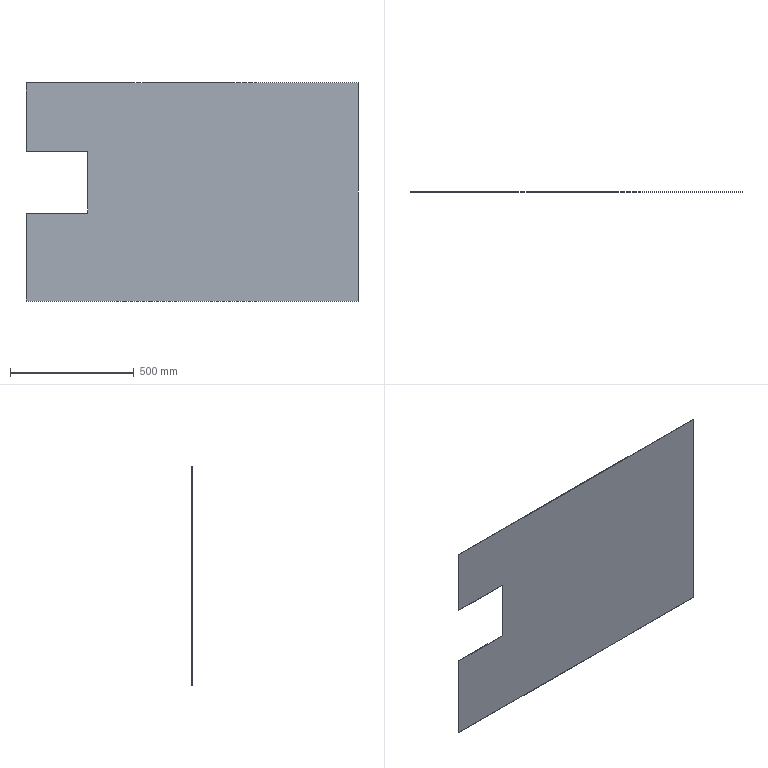Part | STEP file | Sealing plate 1 | 1 solid | 10 faces | box 1340 x 2 x 880 mm | volume 2233400 mm3 | plane 10
STEP:
#1=CARTESIAN_POINT('',(0.,0.,0.));
#2=DIRECTION('',(0.,0.,1.));
#3=DIRECTION('',(1.,0.,0.));
#4=AXIS2_PLACEMENT_3D('',#1,#2,#3);
#5=CARTESIAN_POINT('',(0.,0.,0.));
#6=VERTEX_POINT('',#5);
#7=CARTESIAN_POINT('',(0.,0.,355.));
#8=VERTEX_POINT('',#7);
#9=CARTESIAN_POINT('',(0.,0.,0.));
#10=DIRECTION('',(0.,0.,1.));
#11=VECTOR('',#10,1.);
#12=LINE('',#9,#11);
#13=CARTESIAN_POINT('',(0.,2.,0.));
#14=DIRECTION('',(1.,0.,0.));
#15=DIRECTION('',(0.,0.,-1.));
#16=AXIS2_PLACEMENT_3D('',#13,#14,#15);
#17=PLANE('',#16);
#18=CARTESIAN_POINT('',(0.,-2.));
#19=DIRECTION('',(-1.,0.));
#20=VECTOR('',#19,1.);
#21=LINE('',#18,#20);
#22=(GEOMETRIC_REPRESENTATION_CONTEXT(2)PARAMETRIC_REPRESENTATION_CONTEXT()REPRESENTATION_CONTEXT('',''));
#23=DEFINITIONAL_REPRESENTATION('',(#21),#22);
#24=PCURVE('',#17,#23);
#25=CARTESIAN_POINT('',(0.,0.,0.));
#26=DIRECTION('',(0.,1.,0.));
#27=DIRECTION('',(0.,0.,1.));
#28=AXIS2_PLACEMENT_3D('',#25,#26,#27);
#29=PLANE('',#28);
#30=CARTESIAN_POINT('',(0.,0.));
#31=DIRECTION('',(1.,0.));
#32=VECTOR('',#31,1.);
#33=LINE('',#30,#32);
#34=(GEOMETRIC_REPRESENTATION_CONTEXT(2)PARAMETRIC_REPRESENTATION_CONTEXT()REPRESENTATION_CONTEXT('',''));
#35=DEFINITIONAL_REPRESENTATION('',(#33),#34);
#36=PCURVE('',#29,#35);
#37=SURFACE_CURVE('',#12,(#24,#36),.PCURVE_S1.);
#38=EDGE_CURVE('',#6,#8,#37,.T.);
#39=ORIENTED_EDGE('',*,*,#38,.T.);
#40=CARTESIAN_POINT('',(0.,2.,355.));
#41=VERTEX_POINT('',#40);
#42=CARTESIAN_POINT('',(0.,0.,355.));
#43=DIRECTION('',(0.,1.,0.));
#44=VECTOR('',#43,1.);
#45=LINE('',#42,#44);
#46=CARTESIAN_POINT('',(-355.,-2.));
#47=DIRECTION('',(0.,1.));
#48=VECTOR('',#47,1.);
#49=LINE('',#46,#48);
#50=(GEOMETRIC_REPRESENTATION_CONTEXT(2)PARAMETRIC_REPRESENTATION_CONTEXT()REPRESENTATION_CONTEXT('',''));
#51=DEFINITIONAL_REPRESENTATION('',(#49),#50);
#52=PCURVE('',#17,#51);
#53=CARTESIAN_POINT('',(0.,0.,355.));
#54=DIRECTION('',(0.,0.,-1.));
#55=DIRECTION('',(-1.,0.,0.));
#56=AXIS2_PLACEMENT_3D('',#53,#54,#55);
#57=PLANE('',#56);
#58=CARTESIAN_POINT('',(0.,0.));
#59=DIRECTION('',(0.,1.));
#60=VECTOR('',#59,1.);
#61=LINE('',#58,#60);
#62=(GEOMETRIC_REPRESENTATION_CONTEXT(2)PARAMETRIC_REPRESENTATION_CONTEXT()REPRESENTATION_CONTEXT('',''));
#63=DEFINITIONAL_REPRESENTATION('',(#61),#62);
#64=PCURVE('',#57,#63);
#65=SURFACE_CURVE('',#45,(#52,#64),.PCURVE_S1.);
#66=EDGE_CURVE('',#8,#41,#65,.T.);
#67=ORIENTED_EDGE('',*,*,#66,.T.);
#68=CARTESIAN_POINT('',(0.,2.,0.));
#69=VERTEX_POINT('',#68);
#70=CARTESIAN_POINT('',(0.,2.,0.));
#71=DIRECTION('',(0.,0.,1.));
#72=VECTOR('',#71,1.);
#73=LINE('',#70,#72);
#74=CARTESIAN_POINT('',(0.,0.));
#75=DIRECTION('',(-1.,0.));
#76=VECTOR('',#75,1.);
#77=LINE('',#74,#76);
#78=(GEOMETRIC_REPRESENTATION_CONTEXT(2)PARAMETRIC_REPRESENTATION_CONTEXT()REPRESENTATION_CONTEXT('',''));
#79=DEFINITIONAL_REPRESENTATION('',(#77),#78);
#80=PCURVE('',#17,#79);
#81=CARTESIAN_POINT('',(0.,2.,0.));
#82=DIRECTION('',(0.,1.,0.));
#83=DIRECTION('',(0.,0.,1.));
#84=AXIS2_PLACEMENT_3D('',#81,#82,#83);
#85=PLANE('',#84);
#86=CARTESIAN_POINT('',(0.,0.));
#87=DIRECTION('',(1.,0.));
#88=VECTOR('',#87,1.);
#89=LINE('',#86,#88);
#90=(GEOMETRIC_REPRESENTATION_CONTEXT(2)PARAMETRIC_REPRESENTATION_CONTEXT()REPRESENTATION_CONTEXT('',''));
#91=DEFINITIONAL_REPRESENTATION('',(#89),#90);
#92=PCURVE('',#85,#91);
#93=SURFACE_CURVE('',#73,(#80,#92),.PCURVE_S1.);
#94=EDGE_CURVE('',#69,#41,#93,.T.);
#95=ORIENTED_EDGE('',*,*,#94,.F.);
#96=CARTESIAN_POINT('',(0.,2.,0.));
#97=DIRECTION('',(0.,-1.,0.));
#98=VECTOR('',#97,1.);
#99=LINE('',#96,#98);
#100=CARTESIAN_POINT('',(0.,0.));
#101=DIRECTION('',(0.,-1.));
#102=VECTOR('',#101,1.);
#103=LINE('',#100,#102);
#104=(GEOMETRIC_REPRESENTATION_CONTEXT(2)PARAMETRIC_REPRESENTATION_CONTEXT()REPRESENTATION_CONTEXT('',''));
#105=DEFINITIONAL_REPRESENTATION('',(#103),#104);
#106=PCURVE('',#17,#105);
#107=CARTESIAN_POINT('',(0.,2.,0.));
#108=DIRECTION('',(0.,0.,1.));
#109=DIRECTION('',(1.,0.,0.));
#110=AXIS2_PLACEMENT_3D('',#107,#108,#109);
#111=PLANE('',#110);
#112=CARTESIAN_POINT('',(0.,0.));
#113=DIRECTION('',(0.,-1.));
#114=VECTOR('',#113,1.);
#115=LINE('',#112,#114);
#116=(GEOMETRIC_REPRESENTATION_CONTEXT(2)PARAMETRIC_REPRESENTATION_CONTEXT()REPRESENTATION_CONTEXT('',''));
#117=DEFINITIONAL_REPRESENTATION('',(#115),#116);
#118=PCURVE('',#111,#117);
#119=SURFACE_CURVE('',#99,(#106,#118),.PCURVE_S1.);
#120=EDGE_CURVE('',#69,#6,#119,.T.);
#121=ORIENTED_EDGE('',*,*,#120,.T.);
#122=EDGE_LOOP('',(#39,#67,#95,#121));
#123=FACE_BOUND('',#122,.T.);
#124=ADVANCED_FACE('',(#123),#17,.F.);
#125=CARTESIAN_POINT('',(0.,2.,605.));
#126=VERTEX_POINT('',#125);
#127=CARTESIAN_POINT('',(0.,2.,880.));
#128=VERTEX_POINT('',#127);
#129=CARTESIAN_POINT('',(0.,2.,0.));
#130=DIRECTION('',(0.,0.,1.));
#131=VECTOR('',#130,1.);
#132=LINE('',#129,#131);
#133=CARTESIAN_POINT('',(0.,2.,0.));
#134=DIRECTION('',(1.,0.,0.));
#135=DIRECTION('',(0.,0.,-1.));
#136=AXIS2_PLACEMENT_3D('',#133,#134,#135);
#137=PLANE('',#136);
#138=CARTESIAN_POINT('',(0.,0.));
#139=DIRECTION('',(-1.,0.));
#140=VECTOR('',#139,1.);
#141=LINE('',#138,#140);
#142=(GEOMETRIC_REPRESENTATION_CONTEXT(2)PARAMETRIC_REPRESENTATION_CONTEXT()REPRESENTATION_CONTEXT('',''));
#143=DEFINITIONAL_REPRESENTATION('',(#141),#142);
#144=PCURVE('',#137,#143);
#145=CARTESIAN_POINT('',(0.,0.));
#146=DIRECTION('',(1.,0.));
#147=VECTOR('',#146,1.);
#148=LINE('',#145,#147);
#149=(GEOMETRIC_REPRESENTATION_CONTEXT(2)PARAMETRIC_REPRESENTATION_CONTEXT()REPRESENTATION_CONTEXT('',''));
#150=DEFINITIONAL_REPRESENTATION('',(#148),#149);
#151=PCURVE('',#85,#150);
#152=SURFACE_CURVE('',#132,(#144,#151),.PCURVE_S1.);
#153=EDGE_CURVE('',#126,#128,#152,.T.);
#154=ORIENTED_EDGE('',*,*,#153,.F.);
#155=CARTESIAN_POINT('',(0.,0.,605.));
#156=VERTEX_POINT('',#155);
#157=CARTESIAN_POINT('',(0.,0.,605.));
#158=DIRECTION('',(0.,1.,0.));
#159=VECTOR('',#158,1.);
#160=LINE('',#157,#159);
#161=CARTESIAN_POINT('',(-605.,-2.));
#162=DIRECTION('',(0.,1.));
#163=VECTOR('',#162,1.);
#164=LINE('',#161,#163);
#165=(GEOMETRIC_REPRESENTATION_CONTEXT(2)PARAMETRIC_REPRESENTATION_CONTEXT()REPRESENTATION_CONTEXT('',''));
#166=DEFINITIONAL_REPRESENTATION('',(#164),#165);
#167=PCURVE('',#137,#166);
#168=CARTESIAN_POINT('',(0.,0.,605.));
#169=DIRECTION('',(0.,0.,1.));
#170=DIRECTION('',(1.,0.,0.));
#171=AXIS2_PLACEMENT_3D('',#168,#169,#170);
#172=PLANE('',#171);
#173=CARTESIAN_POINT('',(0.,0.));
#174=DIRECTION('',(0.,1.));
#175=VECTOR('',#174,1.);
#176=LINE('',#173,#175);
#177=(GEOMETRIC_REPRESENTATION_CONTEXT(2)PARAMETRIC_REPRESENTATION_CONTEXT()REPRESENTATION_CONTEXT('',''));
#178=DEFINITIONAL_REPRESENTATION('',(#176),#177);
#179=PCURVE('',#172,#178);
#180=SURFACE_CURVE('',#160,(#167,#179),.PCURVE_S1.);
#181=EDGE_CURVE('',#156,#126,#180,.T.);
#182=ORIENTED_EDGE('',*,*,#181,.F.);
#183=CARTESIAN_POINT('',(0.,0.,880.));
#184=VERTEX_POINT('',#183);
#185=CARTESIAN_POINT('',(0.,0.,0.));
#186=DIRECTION('',(0.,0.,1.));
#187=VECTOR('',#186,1.);
#188=LINE('',#185,#187);
#189=CARTESIAN_POINT('',(0.,-2.));
#190=DIRECTION('',(-1.,0.));
#191=VECTOR('',#190,1.);
#192=LINE('',#189,#191);
#193=(GEOMETRIC_REPRESENTATION_CONTEXT(2)PARAMETRIC_REPRESENTATION_CONTEXT()REPRESENTATION_CONTEXT('',''));
#194=DEFINITIONAL_REPRESENTATION('',(#192),#193);
#195=PCURVE('',#137,#194);
#196=CARTESIAN_POINT('',(0.,0.));
#197=DIRECTION('',(1.,0.));
#198=VECTOR('',#197,1.);
#199=LINE('',#196,#198);
#200=(GEOMETRIC_REPRESENTATION_CONTEXT(2)PARAMETRIC_REPRESENTATION_CONTEXT()REPRESENTATION_CONTEXT('',''));
#201=DEFINITIONAL_REPRESENTATION('',(#199),#200);
#202=PCURVE('',#29,#201);
#203=SURFACE_CURVE('',#188,(#195,#202),.PCURVE_S1.);
#204=EDGE_CURVE('',#156,#184,#203,.T.);
#205=ORIENTED_EDGE('',*,*,#204,.T.);
#206=CARTESIAN_POINT('',(0.,2.,880.));
#207=DIRECTION('',(0.,-1.,0.));
#208=VECTOR('',#207,1.);
#209=LINE('',#206,#208);
#210=CARTESIAN_POINT('',(-880.,0.));
#211=DIRECTION('',(0.,-1.));
#212=VECTOR('',#211,1.);
#213=LINE('',#210,#212);
#214=(GEOMETRIC_REPRESENTATION_CONTEXT(2)PARAMETRIC_REPRESENTATION_CONTEXT()REPRESENTATION_CONTEXT('',''));
#215=DEFINITIONAL_REPRESENTATION('',(#213),#214);
#216=PCURVE('',#137,#215);
#217=CARTESIAN_POINT('',(0.,2.,880.));
#218=DIRECTION('',(0.,0.,-1.));
#219=DIRECTION('',(-1.,0.,0.));
#220=AXIS2_PLACEMENT_3D('',#217,#218,#219);
#221=PLANE('',#220);
#222=CARTESIAN_POINT('',(0.,0.));
#223=DIRECTION('',(0.,-1.));
#224=VECTOR('',#223,1.);
#225=LINE('',#222,#224);
#226=(GEOMETRIC_REPRESENTATION_CONTEXT(2)PARAMETRIC_REPRESENTATION_CONTEXT()REPRESENTATION_CONTEXT('',''));
#227=DEFINITIONAL_REPRESENTATION('',(#225),#226);
#228=PCURVE('',#221,#227);
#229=SURFACE_CURVE('',#209,(#216,#228),.PCURVE_S1.);
#230=EDGE_CURVE('',#128,#184,#229,.T.);
#231=ORIENTED_EDGE('',*,*,#230,.F.);
#232=EDGE_LOOP('',(#154,#182,#205,#231));
#233=FACE_BOUND('',#232,.T.);
#234=ADVANCED_FACE('',(#233),#137,.F.);
#235=CARTESIAN_POINT('',(1340.,0.,880.));
#236=VERTEX_POINT('',#235);
#237=CARTESIAN_POINT('',(0.,0.,880.));
#238=DIRECTION('',(1.,0.,0.));
#239=VECTOR('',#238,1.);
#240=LINE('',#237,#239);
#241=CARTESIAN_POINT('',(0.,-2.));
#242=DIRECTION('',(-1.,0.));
#243=VECTOR('',#242,1.);
#244=LINE('',#241,#243);
#245=(GEOMETRIC_REPRESENTATION_CONTEXT(2)PARAMETRIC_REPRESENTATION_CONTEXT()REPRESENTATION_CONTEXT('',''));
#246=DEFINITIONAL_REPRESENTATION('',(#244),#245);
#247=PCURVE('',#221,#246);
#248=CARTESIAN_POINT('',(880.,0.));
#249=DIRECTION('',(0.,1.));
#250=VECTOR('',#249,1.);
#251=LINE('',#248,#250);
#252=(GEOMETRIC_REPRESENTATION_CONTEXT(2)PARAMETRIC_REPRESENTATION_CONTEXT()REPRESENTATION_CONTEXT('',''));
#253=DEFINITIONAL_REPRESENTATION('',(#251),#252);
#254=PCURVE('',#29,#253);
#255=SURFACE_CURVE('',#240,(#247,#254),.PCURVE_S1.);
#256=EDGE_CURVE('',#184,#236,#255,.T.);
#257=ORIENTED_EDGE('',*,*,#256,.T.);
#258=CARTESIAN_POINT('',(1340.,2.,880.));
#259=VERTEX_POINT('',#258);
#260=CARTESIAN_POINT('',(1340.,2.,880.));
#261=DIRECTION('',(0.,-1.,0.));
#262=VECTOR('',#261,1.);
#263=LINE('',#260,#262);
#264=CARTESIAN_POINT('',(-1340.,0.));
#265=DIRECTION('',(0.,-1.));
#266=VECTOR('',#265,1.);
#267=LINE('',#264,#266);
#268=(GEOMETRIC_REPRESENTATION_CONTEXT(2)PARAMETRIC_REPRESENTATION_CONTEXT()REPRESENTATION_CONTEXT('',''));
#269=DEFINITIONAL_REPRESENTATION('',(#267),#268);
#270=PCURVE('',#221,#269);
#271=CARTESIAN_POINT('',(1340.,2.,0.));
#272=DIRECTION('',(-1.,0.,0.));
#273=DIRECTION('',(0.,0.,1.));
#274=AXIS2_PLACEMENT_3D('',#271,#272,#273);
#275=PLANE('',#274);
#276=CARTESIAN_POINT('',(880.,0.));
#277=DIRECTION('',(0.,-1.));
#278=VECTOR('',#277,1.);
#279=LINE('',#276,#278);
#280=(GEOMETRIC_REPRESENTATION_CONTEXT(2)PARAMETRIC_REPRESENTATION_CONTEXT()REPRESENTATION_CONTEXT('',''));
#281=DEFINITIONAL_REPRESENTATION('',(#279),#280);
#282=PCURVE('',#275,#281);
#283=SURFACE_CURVE('',#263,(#270,#282),.PCURVE_S1.);
#284=EDGE_CURVE('',#259,#236,#283,.T.);
#285=ORIENTED_EDGE('',*,*,#284,.F.);
#286=CARTESIAN_POINT('',(0.,2.,880.));
#287=DIRECTION('',(1.,0.,0.));
#288=VECTOR('',#287,1.);
#289=LINE('',#286,#288);
#290=CARTESIAN_POINT('',(0.,0.));
#291=DIRECTION('',(-1.,0.));
#292=VECTOR('',#291,1.);
#293=LINE('',#290,#292);
#294=(GEOMETRIC_REPRESENTATION_CONTEXT(2)PARAMETRIC_REPRESENTATION_CONTEXT()REPRESENTATION_CONTEXT('',''));
#295=DEFINITIONAL_REPRESENTATION('',(#293),#294);
#296=PCURVE('',#221,#295);
#297=CARTESIAN_POINT('',(880.,0.));
#298=DIRECTION('',(0.,1.));
#299=VECTOR('',#298,1.);
#300=LINE('',#297,#299);
#301=(GEOMETRIC_REPRESENTATION_CONTEXT(2)PARAMETRIC_REPRESENTATION_CONTEXT()REPRESENTATION_CONTEXT('',''));
#302=DEFINITIONAL_REPRESENTATION('',(#300),#301);
#303=PCURVE('',#85,#302);
#304=SURFACE_CURVE('',#289,(#296,#303),.PCURVE_S1.);
#305=EDGE_CURVE('',#128,#259,#304,.T.);
#306=ORIENTED_EDGE('',*,*,#305,.F.);
#307=ORIENTED_EDGE('',*,*,#230,.T.);
#308=EDGE_LOOP('',(#257,#285,#306,#307));
#309=FACE_BOUND('',#308,.T.);
#310=ADVANCED_FACE('',(#309),#221,.F.);
#311=CARTESIAN_POINT('',(1340.,0.,0.));
#312=VERTEX_POINT('',#311);
#313=CARTESIAN_POINT('',(1340.,0.,0.));
#314=DIRECTION('',(0.,0.,-1.));
#315=VECTOR('',#314,1.);
#316=LINE('',#313,#315);
#317=CARTESIAN_POINT('',(0.,-2.));
#318=DIRECTION('',(-1.,0.));
#319=VECTOR('',#318,1.);
#320=LINE('',#317,#319);
#321=(GEOMETRIC_REPRESENTATION_CONTEXT(2)PARAMETRIC_REPRESENTATION_CONTEXT()REPRESENTATION_CONTEXT('',''));
#322=DEFINITIONAL_REPRESENTATION('',(#320),#321);
#323=PCURVE('',#275,#322);
#324=CARTESIAN_POINT('',(0.,1340.));
#325=DIRECTION('',(-1.,0.));
#326=VECTOR('',#325,1.);
#327=LINE('',#324,#326);
#328=(GEOMETRIC_REPRESENTATION_CONTEXT(2)PARAMETRIC_REPRESENTATION_CONTEXT()REPRESENTATION_CONTEXT('',''));
#329=DEFINITIONAL_REPRESENTATION('',(#327),#328);
#330=PCURVE('',#29,#329);
#331=SURFACE_CURVE('',#316,(#323,#330),.PCURVE_S1.);
#332=EDGE_CURVE('',#236,#312,#331,.T.);
#333=ORIENTED_EDGE('',*,*,#332,.T.);
#334=CARTESIAN_POINT('',(1340.,2.,0.));
#335=VERTEX_POINT('',#334);
#336=CARTESIAN_POINT('',(1340.,2.,0.));
#337=DIRECTION('',(0.,-1.,0.));
#338=VECTOR('',#337,1.);
#339=LINE('',#336,#338);
#340=CARTESIAN_POINT('',(0.,0.));
#341=DIRECTION('',(0.,-1.));
#342=VECTOR('',#341,1.);
#343=LINE('',#340,#342);
#344=(GEOMETRIC_REPRESENTATION_CONTEXT(2)PARAMETRIC_REPRESENTATION_CONTEXT()REPRESENTATION_CONTEXT('',''));
#345=DEFINITIONAL_REPRESENTATION('',(#343),#344);
#346=PCURVE('',#275,#345);
#347=CARTESIAN_POINT('',(1340.,0.));
#348=DIRECTION('',(0.,-1.));
#349=VECTOR('',#348,1.);
#350=LINE('',#347,#349);
#351=(GEOMETRIC_REPRESENTATION_CONTEXT(2)PARAMETRIC_REPRESENTATION_CONTEXT()REPRESENTATION_CONTEXT('',''));
#352=DEFINITIONAL_REPRESENTATION('',(#350),#351);
#353=PCURVE('',#111,#352);
#354=SURFACE_CURVE('',#339,(#346,#353),.PCURVE_S1.);
#355=EDGE_CURVE('',#335,#312,#354,.T.);
#356=ORIENTED_EDGE('',*,*,#355,.F.);
#357=CARTESIAN_POINT('',(1340.,2.,0.));
#358=DIRECTION('',(0.,0.,-1.));
#359=VECTOR('',#358,1.);
#360=LINE('',#357,#359);
#361=CARTESIAN_POINT('',(0.,0.));
#362=DIRECTION('',(-1.,0.));
#363=VECTOR('',#362,1.);
#364=LINE('',#361,#363);
#365=(GEOMETRIC_REPRESENTATION_CONTEXT(2)PARAMETRIC_REPRESENTATION_CONTEXT()REPRESENTATION_CONTEXT('',''));
#366=DEFINITIONAL_REPRESENTATION('',(#364),#365);
#367=PCURVE('',#275,#366);
#368=CARTESIAN_POINT('',(0.,1340.));
#369=DIRECTION('',(-1.,0.));
#370=VECTOR('',#369,1.);
#371=LINE('',#368,#370);
#372=(GEOMETRIC_REPRESENTATION_CONTEXT(2)PARAMETRIC_REPRESENTATION_CONTEXT()REPRESENTATION_CONTEXT('',''));
#373=DEFINITIONAL_REPRESENTATION('',(#371),#372);
#374=PCURVE('',#85,#373);
#375=SURFACE_CURVE('',#360,(#367,#374),.PCURVE_S1.);
#376=EDGE_CURVE('',#259,#335,#375,.T.);
#377=ORIENTED_EDGE('',*,*,#376,.F.);
#378=ORIENTED_EDGE('',*,*,#284,.T.);
#379=EDGE_LOOP('',(#333,#356,#377,#378));
#380=FACE_BOUND('',#379,.T.);
#381=ADVANCED_FACE('',(#380),#275,.F.);
#382=CARTESIAN_POINT('',(0.,0.,0.));
#383=DIRECTION('',(-1.,0.,0.));
#384=VECTOR('',#383,1.);
#385=LINE('',#382,#384);
#386=CARTESIAN_POINT('',(0.,-2.));
#387=DIRECTION('',(-1.,0.));
#388=VECTOR('',#387,1.);
#389=LINE('',#386,#388);
#390=(GEOMETRIC_REPRESENTATION_CONTEXT(2)PARAMETRIC_REPRESENTATION_CONTEXT()REPRESENTATION_CONTEXT('',''));
#391=DEFINITIONAL_REPRESENTATION('',(#389),#390);
#392=PCURVE('',#111,#391);
#393=CARTESIAN_POINT('',(0.,0.));
#394=DIRECTION('',(0.,-1.));
#395=VECTOR('',#394,1.);
#396=LINE('',#393,#395);
#397=(GEOMETRIC_REPRESENTATION_CONTEXT(2)PARAMETRIC_REPRESENTATION_CONTEXT()REPRESENTATION_CONTEXT('',''));
#398=DEFINITIONAL_REPRESENTATION('',(#396),#397);
#399=PCURVE('',#29,#398);
#400=SURFACE_CURVE('',#385,(#392,#399),.PCURVE_S1.);
#401=EDGE_CURVE('',#312,#6,#400,.T.);
#402=ORIENTED_EDGE('',*,*,#401,.T.);
#403=ORIENTED_EDGE('',*,*,#120,.F.);
#404=CARTESIAN_POINT('',(0.,2.,0.));
#405=DIRECTION('',(-1.,0.,0.));
#406=VECTOR('',#405,1.);
#407=LINE('',#404,#406);
#408=CARTESIAN_POINT('',(0.,0.));
#409=DIRECTION('',(-1.,0.));
#410=VECTOR('',#409,1.);
#411=LINE('',#408,#410);
#412=(GEOMETRIC_REPRESENTATION_CONTEXT(2)PARAMETRIC_REPRESENTATION_CONTEXT()REPRESENTATION_CONTEXT('',''));
#413=DEFINITIONAL_REPRESENTATION('',(#411),#412);
#414=PCURVE('',#111,#413);
#415=CARTESIAN_POINT('',(0.,0.));
#416=DIRECTION('',(0.,-1.));
#417=VECTOR('',#416,1.);
#418=LINE('',#415,#417);
#419=(GEOMETRIC_REPRESENTATION_CONTEXT(2)PARAMETRIC_REPRESENTATION_CONTEXT()REPRESENTATION_CONTEXT('',''));
#420=DEFINITIONAL_REPRESENTATION('',(#418),#419);
#421=PCURVE('',#85,#420);
#422=SURFACE_CURVE('',#407,(#414,#421),.PCURVE_S1.);
#423=EDGE_CURVE('',#335,#69,#422,.T.);
#424=ORIENTED_EDGE('',*,*,#423,.F.);
#425=ORIENTED_EDGE('',*,*,#355,.T.);
#426=EDGE_LOOP('',(#402,#403,#424,#425));
#427=FACE_BOUND('',#426,.T.);
#428=ADVANCED_FACE('',(#427),#111,.F.);
#429=CARTESIAN_POINT('',(250.,2.,355.));
#430=VERTEX_POINT('',#429);
#431=CARTESIAN_POINT('',(0.,2.,355.));
#432=DIRECTION('',(-1.,0.,0.));
#433=VECTOR('',#432,1.);
#434=LINE('',#431,#433);
#435=CARTESIAN_POINT('',(355.,0.));
#436=DIRECTION('',(0.,-1.));
#437=VECTOR('',#436,1.);
#438=LINE('',#435,#437);
#439=(GEOMETRIC_REPRESENTATION_CONTEXT(2)PARAMETRIC_REPRESENTATION_CONTEXT()REPRESENTATION_CONTEXT('',''));
#440=DEFINITIONAL_REPRESENTATION('',(#438),#439);
#441=PCURVE('',#85,#440);
#442=CARTESIAN_POINT('',(0.,2.));
#443=DIRECTION('',(1.,0.));
#444=VECTOR('',#443,1.);
#445=LINE('',#442,#444);
#446=(GEOMETRIC_REPRESENTATION_CONTEXT(2)PARAMETRIC_REPRESENTATION_CONTEXT()REPRESENTATION_CONTEXT('',''));
#447=DEFINITIONAL_REPRESENTATION('',(#445),#446);
#448=PCURVE('',#57,#447);
#449=SURFACE_CURVE('',#434,(#441,#448),.PCURVE_S1.);
#450=EDGE_CURVE('',#430,#41,#449,.T.);
#451=ORIENTED_EDGE('',*,*,#450,.F.);
#452=CARTESIAN_POINT('',(250.,2.,605.));
#453=VERTEX_POINT('',#452);
#454=CARTESIAN_POINT('',(250.,2.,605.));
#455=DIRECTION('',(0.,0.,-1.));
#456=VECTOR('',#455,1.);
#457=LINE('',#454,#456);
#458=CARTESIAN_POINT('',(605.,250.));
#459=DIRECTION('',(-1.,0.));
#460=VECTOR('',#459,1.);
#461=LINE('',#458,#460);
#462=(GEOMETRIC_REPRESENTATION_CONTEXT(2)PARAMETRIC_REPRESENTATION_CONTEXT()REPRESENTATION_CONTEXT('',''));
#463=DEFINITIONAL_REPRESENTATION('',(#461),#462);
#464=PCURVE('',#85,#463);
#465=CARTESIAN_POINT('',(250.,0.,605.));
#466=DIRECTION('',(1.,0.,0.));
#467=DIRECTION('',(0.,0.,-1.));
#468=AXIS2_PLACEMENT_3D('',#465,#466,#467);
#469=PLANE('',#468);
#470=CARTESIAN_POINT('',(0.,2.));
#471=DIRECTION('',(1.,0.));
#472=VECTOR('',#471,1.);
#473=LINE('',#470,#472);
#474=(GEOMETRIC_REPRESENTATION_CONTEXT(2)PARAMETRIC_REPRESENTATION_CONTEXT()REPRESENTATION_CONTEXT('',''));
#475=DEFINITIONAL_REPRESENTATION('',(#473),#474);
#476=PCURVE('',#469,#475);
#477=SURFACE_CURVE('',#457,(#464,#476),.PCURVE_S1.);
#478=EDGE_CURVE('',#453,#430,#477,.T.);
#479=ORIENTED_EDGE('',*,*,#478,.F.);
#480=CARTESIAN_POINT('',(0.,2.,605.));
#481=DIRECTION('',(1.,0.,0.));
#482=VECTOR('',#481,1.);
#483=LINE('',#480,#482);
#484=CARTESIAN_POINT('',(605.,0.));
#485=DIRECTION('',(0.,1.));
#486=VECTOR('',#485,1.);
#487=LINE('',#484,#486);
#488=(GEOMETRIC_REPRESENTATION_CONTEXT(2)PARAMETRIC_REPRESENTATION_CONTEXT()REPRESENTATION_CONTEXT('',''));
#489=DEFINITIONAL_REPRESENTATION('',(#487),#488);
#490=PCURVE('',#85,#489);
#491=CARTESIAN_POINT('',(0.,2.));
#492=DIRECTION('',(1.,0.));
#493=VECTOR('',#492,1.);
#494=LINE('',#491,#493);
#495=(GEOMETRIC_REPRESENTATION_CONTEXT(2)PARAMETRIC_REPRESENTATION_CONTEXT()REPRESENTATION_CONTEXT('',''));
#496=DEFINITIONAL_REPRESENTATION('',(#494),#495);
#497=PCURVE('',#172,#496);
#498=SURFACE_CURVE('',#483,(#490,#497),.PCURVE_S1.);
#499=EDGE_CURVE('',#126,#453,#498,.T.);
#500=ORIENTED_EDGE('',*,*,#499,.F.);
#501=ORIENTED_EDGE('',*,*,#153,.T.);
#502=ORIENTED_EDGE('',*,*,#305,.T.);
#503=ORIENTED_EDGE('',*,*,#376,.T.);
#504=ORIENTED_EDGE('',*,*,#423,.T.);
#505=ORIENTED_EDGE('',*,*,#94,.T.);
#506=EDGE_LOOP('',(#451,#479,#500,#501,#502,#503,#504,#505));
#507=FACE_BOUND('',#506,.T.);
#508=ADVANCED_FACE('',(#507),#85,.T.);
#509=CARTESIAN_POINT('',(250.,0.,605.));
#510=VERTEX_POINT('',#509);
#511=CARTESIAN_POINT('',(250.,0.,355.));
#512=VERTEX_POINT('',#511);
#513=CARTESIAN_POINT('',(250.,0.,605.));
#514=DIRECTION('',(0.,0.,-1.));
#515=VECTOR('',#514,1.);
#516=LINE('',#513,#515);
#517=CARTESIAN_POINT('',(605.,250.));
#518=DIRECTION('',(-1.,0.));
#519=VECTOR('',#518,1.);
#520=LINE('',#517,#519);
#521=(GEOMETRIC_REPRESENTATION_CONTEXT(2)PARAMETRIC_REPRESENTATION_CONTEXT()REPRESENTATION_CONTEXT('',''));
#522=DEFINITIONAL_REPRESENTATION('',(#520),#521);
#523=PCURVE('',#29,#522);
#524=CARTESIAN_POINT('',(0.,0.));
#525=DIRECTION('',(1.,0.));
#526=VECTOR('',#525,1.);
#527=LINE('',#524,#526);
#528=(GEOMETRIC_REPRESENTATION_CONTEXT(2)PARAMETRIC_REPRESENTATION_CONTEXT()REPRESENTATION_CONTEXT('',''));
#529=DEFINITIONAL_REPRESENTATION('',(#527),#528);
#530=PCURVE('',#469,#529);
#531=SURFACE_CURVE('',#516,(#523,#530),.PCURVE_S1.);
#532=EDGE_CURVE('',#510,#512,#531,.T.);
#533=ORIENTED_EDGE('',*,*,#532,.T.);
#534=CARTESIAN_POINT('',(0.,0.,355.));
#535=DIRECTION('',(-1.,0.,0.));
#536=VECTOR('',#535,1.);
#537=LINE('',#534,#536);
#538=CARTESIAN_POINT('',(355.,0.));
#539=DIRECTION('',(0.,-1.));
#540=VECTOR('',#539,1.);
#541=LINE('',#538,#540);
#542=(GEOMETRIC_REPRESENTATION_CONTEXT(2)PARAMETRIC_REPRESENTATION_CONTEXT()REPRESENTATION_CONTEXT('',''));
#543=DEFINITIONAL_REPRESENTATION('',(#541),#542);
#544=PCURVE('',#29,#543);
#545=CARTESIAN_POINT('',(0.,0.));
#546=DIRECTION('',(1.,0.));
#547=VECTOR('',#546,1.);
#548=LINE('',#545,#547);
#549=(GEOMETRIC_REPRESENTATION_CONTEXT(2)PARAMETRIC_REPRESENTATION_CONTEXT()REPRESENTATION_CONTEXT('',''));
#550=DEFINITIONAL_REPRESENTATION('',(#548),#549);
#551=PCURVE('',#57,#550);
#552=SURFACE_CURVE('',#537,(#544,#551),.PCURVE_S1.);
#553=EDGE_CURVE('',#512,#8,#552,.T.);
#554=ORIENTED_EDGE('',*,*,#553,.T.);
#555=ORIENTED_EDGE('',*,*,#38,.F.);
#556=ORIENTED_EDGE('',*,*,#401,.F.);
#557=ORIENTED_EDGE('',*,*,#332,.F.);
#558=ORIENTED_EDGE('',*,*,#256,.F.);
#559=ORIENTED_EDGE('',*,*,#204,.F.);
#560=CARTESIAN_POINT('',(0.,0.,605.));
#561=DIRECTION('',(1.,0.,0.));
#562=VECTOR('',#561,1.);
#563=LINE('',#560,#562);
#564=CARTESIAN_POINT('',(605.,0.));
#565=DIRECTION('',(0.,1.));
#566=VECTOR('',#565,1.);
#567=LINE('',#564,#566);
#568=(GEOMETRIC_REPRESENTATION_CONTEXT(2)PARAMETRIC_REPRESENTATION_CONTEXT()REPRESENTATION_CONTEXT('',''));
#569=DEFINITIONAL_REPRESENTATION('',(#567),#568);
#570=PCURVE('',#29,#569);
#571=CARTESIAN_POINT('',(0.,0.));
#572=DIRECTION('',(1.,0.));
#573=VECTOR('',#572,1.);
#574=LINE('',#571,#573);
#575=(GEOMETRIC_REPRESENTATION_CONTEXT(2)PARAMETRIC_REPRESENTATION_CONTEXT()REPRESENTATION_CONTEXT('',''));
#576=DEFINITIONAL_REPRESENTATION('',(#574),#575);
#577=PCURVE('',#172,#576);
#578=SURFACE_CURVE('',#563,(#570,#577),.PCURVE_S1.);
#579=EDGE_CURVE('',#156,#510,#578,.T.);
#580=ORIENTED_EDGE('',*,*,#579,.T.);
#581=EDGE_LOOP('',(#533,#554,#555,#556,#557,#558,#559,#580));
#582=FACE_BOUND('',#581,.T.);
#583=ADVANCED_FACE('',(#582),#29,.F.);
#584=ORIENTED_EDGE('',*,*,#450,.T.);
#585=ORIENTED_EDGE('',*,*,#66,.F.);
#586=ORIENTED_EDGE('',*,*,#553,.F.);
#587=CARTESIAN_POINT('',(250.,0.,355.));
#588=DIRECTION('',(0.,1.,0.));
#589=VECTOR('',#588,1.);
#590=LINE('',#587,#589);
#591=CARTESIAN_POINT('',(-250.,0.));
#592=DIRECTION('',(0.,1.));
#593=VECTOR('',#592,1.);
#594=LINE('',#591,#593);
#595=(GEOMETRIC_REPRESENTATION_CONTEXT(2)PARAMETRIC_REPRESENTATION_CONTEXT()REPRESENTATION_CONTEXT('',''));
#596=DEFINITIONAL_REPRESENTATION('',(#594),#595);
#597=PCURVE('',#57,#596);
#598=CARTESIAN_POINT('',(250.,0.));
#599=DIRECTION('',(0.,1.));
#600=VECTOR('',#599,1.);
#601=LINE('',#598,#600);
#602=(GEOMETRIC_REPRESENTATION_CONTEXT(2)PARAMETRIC_REPRESENTATION_CONTEXT()REPRESENTATION_CONTEXT('',''));
#603=DEFINITIONAL_REPRESENTATION('',(#601),#602);
#604=PCURVE('',#469,#603);
#605=SURFACE_CURVE('',#590,(#597,#604),.PCURVE_S1.);
#606=EDGE_CURVE('',#512,#430,#605,.T.);
#607=ORIENTED_EDGE('',*,*,#606,.T.);
#608=EDGE_LOOP('',(#584,#585,#586,#607));
#609=FACE_BOUND('',#608,.T.);
#610=ADVANCED_FACE('',(#609),#57,.F.);
#611=ORIENTED_EDGE('',*,*,#478,.T.);
#612=ORIENTED_EDGE('',*,*,#606,.F.);
#613=ORIENTED_EDGE('',*,*,#532,.F.);
#614=CARTESIAN_POINT('',(250.,0.,605.));
#615=DIRECTION('',(0.,1.,0.));
#616=VECTOR('',#615,1.);
#617=LINE('',#614,#616);
#618=CARTESIAN_POINT('',(0.,0.));
#619=DIRECTION('',(0.,1.));
#620=VECTOR('',#619,1.);
#621=LINE('',#618,#620);
#622=(GEOMETRIC_REPRESENTATION_CONTEXT(2)PARAMETRIC_REPRESENTATION_CONTEXT()REPRESENTATION_CONTEXT('',''));
#623=DEFINITIONAL_REPRESENTATION('',(#621),#622);
#624=PCURVE('',#469,#623);
#625=CARTESIAN_POINT('',(250.,0.));
#626=DIRECTION('',(0.,1.));
#627=VECTOR('',#626,1.);
#628=LINE('',#625,#627);
#629=(GEOMETRIC_REPRESENTATION_CONTEXT(2)PARAMETRIC_REPRESENTATION_CONTEXT()REPRESENTATION_CONTEXT('',''));
#630=DEFINITIONAL_REPRESENTATION('',(#628),#629);
#631=PCURVE('',#172,#630);
#632=SURFACE_CURVE('',#617,(#624,#631),.PCURVE_S1.);
#633=EDGE_CURVE('',#510,#453,#632,.T.);
#634=ORIENTED_EDGE('',*,*,#633,.T.);
#635=EDGE_LOOP('',(#611,#612,#613,#634));
#636=FACE_BOUND('',#635,.T.);
#637=ADVANCED_FACE('',(#636),#469,.F.);
#638=ORIENTED_EDGE('',*,*,#499,.T.);
#639=ORIENTED_EDGE('',*,*,#633,.F.);
#640=ORIENTED_EDGE('',*,*,#579,.F.);
#641=ORIENTED_EDGE('',*,*,#181,.T.);
#642=EDGE_LOOP('',(#638,#639,#640,#641));
#643=FACE_BOUND('',#642,.T.);
#644=ADVANCED_FACE('',(#643),#172,.F.);
#645=CLOSED_SHELL('',(#124,#234,#310,#381,#428,#508,#583,#610,#637,#644));
#646=MANIFOLD_SOLID_BREP('',#645);
#647=(LENGTH_UNIT()NAMED_UNIT(*)SI_UNIT(.MILLI.,.METRE.));
#648=UNCERTAINTY_MEASURE_WITH_UNIT(LENGTH_MEASURE(0.0000001),#647,'','');
#649=(NAMED_UNIT(*)PLANE_ANGLE_UNIT()SI_UNIT($,.RADIAN.));
#650=(NAMED_UNIT(*)SI_UNIT($,.STERADIAN.)SOLID_ANGLE_UNIT());
#651=(GEOMETRIC_REPRESENTATION_CONTEXT(3)GLOBAL_UNCERTAINTY_ASSIGNED_CONTEXT((#648))GLOBAL_UNIT_ASSIGNED_CONTEXT((#647,#649,#650))REPRESENTATION_CONTEXT('',''));
#652=ADVANCED_BREP_SHAPE_REPRESENTATION('',(#4,#646),#651);